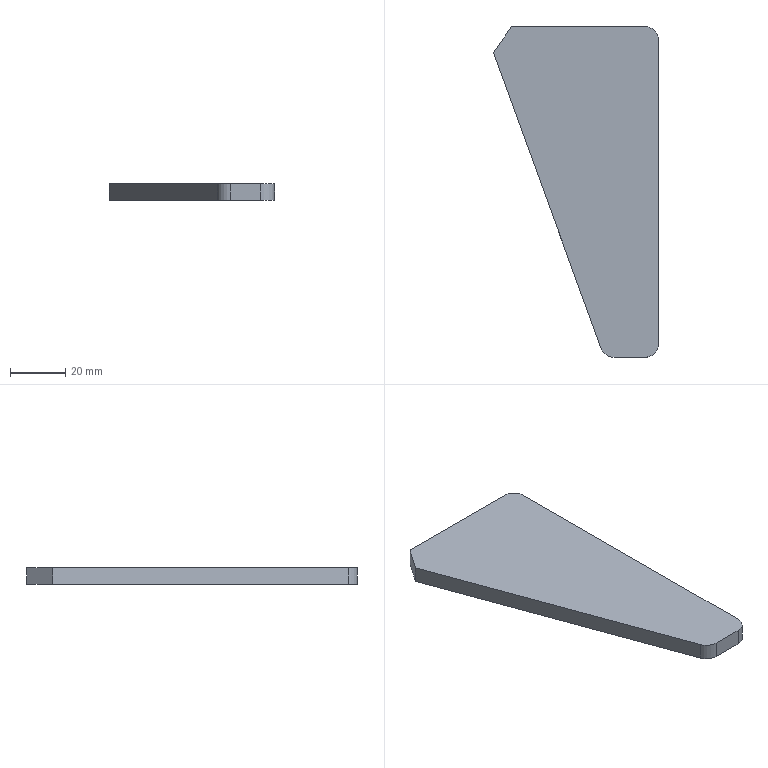Part | SolidWorks | features FlatPattern 1, SMBaseFlange 1, SheetMetal 1 | 1 solid | 10 faces | box 59.933 x 120 x 6 mm | volume 29531 mm3 | plane 7 | cylinder 3 | commonest cylinder face diameters 10 x3
STEP:
#1=CARTESIAN_POINT('',(295.827,-93.574,0.));
#2=VERTEX_POINT('',#1);
#3=CARTESIAN_POINT('',(290.827,-88.574,0.));
#4=VERTEX_POINT('',#3);
#5=CARTESIAN_POINT('',(290.827,-93.574,0.));
#6=DIRECTION('',(0.,0.,1.));
#7=DIRECTION('',(-1.,0.,0.));
#8=AXIS2_PLACEMENT_3D('',#5,#6,#7);
#9=CIRCLE('',#8,5.);
#10=EDGE_CURVE('',#2,#4,#9,.T.);
#11=ORIENTED_EDGE('',*,*,#10,.F.);
#12=CARTESIAN_POINT('',(295.827,-93.574,-6.));
#13=VERTEX_POINT('',#12);
#14=CARTESIAN_POINT('',(295.827,-93.574,-6.));
#15=DIRECTION('',(0.,0.,1.));
#16=VECTOR('',#15,1000.);
#17=LINE('',#14,#16);
#18=EDGE_CURVE('',#13,#2,#17,.T.);
#19=ORIENTED_EDGE('',*,*,#18,.F.);
#20=CARTESIAN_POINT('',(290.827,-88.574,-6.));
#21=VERTEX_POINT('',#20);
#22=CARTESIAN_POINT('',(290.827,-93.574,-6.));
#23=DIRECTION('',(0.,0.,1.));
#24=DIRECTION('',(-1.,0.,0.));
#25=AXIS2_PLACEMENT_3D('',#22,#23,#24);
#26=CIRCLE('',#25,5.);
#27=EDGE_CURVE('',#13,#21,#26,.T.);
#28=ORIENTED_EDGE('',*,*,#27,.T.);
#29=CARTESIAN_POINT('',(290.827,-88.574,-6.));
#30=DIRECTION('',(0.,0.,1.));
#31=VECTOR('',#30,1000.);
#32=LINE('',#29,#31);
#33=EDGE_CURVE('',#21,#4,#32,.T.);
#34=ORIENTED_EDGE('',*,*,#33,.T.);
#35=EDGE_LOOP('',(#11,#19,#28,#34));
#36=FACE_OUTER_BOUND('',#35,.T.);
#37=CARTESIAN_POINT('',(290.827,-93.574,-6.));
#38=DIRECTION('',(0.,0.,1.));
#39=DIRECTION('',(1.,0.,0.));
#40=AXIS2_PLACEMENT_3D('',#37,#38,#39);
#41=CYLINDRICAL_SURFACE('',#40,5.);
#42=ADVANCED_FACE('',(#36),#41,.T.);
#43=CARTESIAN_POINT('',(295.827,-203.574,0.));
#44=VERTEX_POINT('',#43);
#45=CARTESIAN_POINT('',(295.827,-93.574,0.));
#46=DIRECTION('',(0.,1.,0.));
#47=VECTOR('',#46,1000.);
#48=LINE('',#45,#47);
#49=EDGE_CURVE('',#44,#2,#48,.T.);
#50=ORIENTED_EDGE('',*,*,#49,.F.);
#51=CARTESIAN_POINT('',(295.827,-203.574,-6.));
#52=VERTEX_POINT('',#51);
#53=CARTESIAN_POINT('',(295.827,-203.574,-6.));
#54=DIRECTION('',(0.,0.,1.));
#55=VECTOR('',#54,1000.);
#56=LINE('',#53,#55);
#57=EDGE_CURVE('',#52,#44,#56,.T.);
#58=ORIENTED_EDGE('',*,*,#57,.F.);
#59=CARTESIAN_POINT('',(295.827,-93.574,-6.));
#60=DIRECTION('',(0.,1.,0.));
#61=VECTOR('',#60,1000.);
#62=LINE('',#59,#61);
#63=EDGE_CURVE('',#52,#13,#62,.T.);
#64=ORIENTED_EDGE('',*,*,#63,.T.);
#65=ORIENTED_EDGE('',*,*,#18,.T.);
#66=EDGE_LOOP('',(#50,#58,#64,#65));
#67=FACE_OUTER_BOUND('',#66,.T.);
#68=CARTESIAN_POINT('',(295.827,-93.574,-6.));
#69=DIRECTION('',(1.,0.,0.));
#70=DIRECTION('',(0.,0.,-1.));
#71=AXIS2_PLACEMENT_3D('',#68,#69,#70);
#72=PLANE('',#71);
#73=ADVANCED_FACE('',(#67),#72,.T.);
#74=CARTESIAN_POINT('',(290.827,-208.574,0.));
#75=VERTEX_POINT('',#74);
#76=CARTESIAN_POINT('',(290.827,-203.574,0.));
#77=DIRECTION('',(0.,0.,1.));
#78=DIRECTION('',(-1.,0.,0.));
#79=AXIS2_PLACEMENT_3D('',#76,#77,#78);
#80=CIRCLE('',#79,5.);
#81=EDGE_CURVE('',#75,#44,#80,.T.);
#82=ORIENTED_EDGE('',*,*,#81,.F.);
#83=CARTESIAN_POINT('',(290.827,-208.574,-6.));
#84=VERTEX_POINT('',#83);
#85=CARTESIAN_POINT('',(290.827,-208.574,-6.));
#86=DIRECTION('',(0.,0.,1.));
#87=VECTOR('',#86,1000.);
#88=LINE('',#85,#87);
#89=EDGE_CURVE('',#84,#75,#88,.T.);
#90=ORIENTED_EDGE('',*,*,#89,.F.);
#91=CARTESIAN_POINT('',(290.827,-203.574,-6.));
#92=DIRECTION('',(0.,0.,1.));
#93=DIRECTION('',(-1.,0.,0.));
#94=AXIS2_PLACEMENT_3D('',#91,#92,#93);
#95=CIRCLE('',#94,5.);
#96=EDGE_CURVE('',#84,#52,#95,.T.);
#97=ORIENTED_EDGE('',*,*,#96,.T.);
#98=ORIENTED_EDGE('',*,*,#57,.T.);
#99=EDGE_LOOP('',(#82,#90,#97,#98));
#100=FACE_OUTER_BOUND('',#99,.T.);
#101=CARTESIAN_POINT('',(290.827,-203.574,-6.));
#102=DIRECTION('',(0.,0.,1.));
#103=DIRECTION('',(1.,0.,0.));
#104=AXIS2_PLACEMENT_3D('',#101,#102,#103);
#105=CYLINDRICAL_SURFACE('',#104,5.);
#106=ADVANCED_FACE('',(#100),#105,.T.);
#107=CARTESIAN_POINT('',(279.652,-208.574,0.));
#108=VERTEX_POINT('',#107);
#109=CARTESIAN_POINT('',(290.827,-208.574,0.));
#110=DIRECTION('',(1.,0.,0.));
#111=VECTOR('',#110,1000.);
#112=LINE('',#109,#111);
#113=EDGE_CURVE('',#108,#75,#112,.T.);
#114=ORIENTED_EDGE('',*,*,#113,.F.);
#115=CARTESIAN_POINT('',(279.652,-208.574,-6.));
#116=VERTEX_POINT('',#115);
#117=CARTESIAN_POINT('',(279.652,-208.574,-6.));
#118=DIRECTION('',(0.,0.,1.));
#119=VECTOR('',#118,1000.);
#120=LINE('',#117,#119);
#121=EDGE_CURVE('',#116,#108,#120,.T.);
#122=ORIENTED_EDGE('',*,*,#121,.F.);
#123=CARTESIAN_POINT('',(290.827,-208.574,-6.));
#124=DIRECTION('',(1.,0.,0.));
#125=VECTOR('',#124,1000.);
#126=LINE('',#123,#125);
#127=EDGE_CURVE('',#116,#84,#126,.T.);
#128=ORIENTED_EDGE('',*,*,#127,.T.);
#129=ORIENTED_EDGE('',*,*,#89,.T.);
#130=EDGE_LOOP('',(#114,#122,#128,#129));
#131=FACE_OUTER_BOUND('',#130,.T.);
#132=CARTESIAN_POINT('',(290.827,-208.574,-6.));
#133=DIRECTION('',(0.,-1.,0.));
#134=DIRECTION('',(0.,0.,-1.));
#135=AXIS2_PLACEMENT_3D('',#132,#133,#134);
#136=PLANE('',#135);
#137=ADVANCED_FACE('',(#131),#136,.T.);
#138=CARTESIAN_POINT('',(274.953,-205.284,0.));
#139=VERTEX_POINT('',#138);
#140=CARTESIAN_POINT('',(279.652,-203.574,0.));
#141=DIRECTION('',(0.,0.,1.));
#142=DIRECTION('',(1.,0.,0.));
#143=AXIS2_PLACEMENT_3D('',#140,#141,#142);
#144=CIRCLE('',#143,5.);
#145=EDGE_CURVE('',#139,#108,#144,.T.);
#146=ORIENTED_EDGE('',*,*,#145,.F.);
#147=CARTESIAN_POINT('',(274.953,-205.284,-6.));
#148=VERTEX_POINT('',#147);
#149=CARTESIAN_POINT('',(274.953,-205.284,-6.));
#150=DIRECTION('',(0.,0.,1.));
#151=VECTOR('',#150,1000.);
#152=LINE('',#149,#151);
#153=EDGE_CURVE('',#148,#139,#152,.T.);
#154=ORIENTED_EDGE('',*,*,#153,.F.);
#155=CARTESIAN_POINT('',(279.652,-203.574,-6.));
#156=DIRECTION('',(0.,0.,1.));
#157=DIRECTION('',(1.,0.,0.));
#158=AXIS2_PLACEMENT_3D('',#155,#156,#157);
#159=CIRCLE('',#158,5.);
#160=EDGE_CURVE('',#148,#116,#159,.T.);
#161=ORIENTED_EDGE('',*,*,#160,.T.);
#162=ORIENTED_EDGE('',*,*,#121,.T.);
#163=EDGE_LOOP('',(#146,#154,#161,#162));
#164=FACE_OUTER_BOUND('',#163,.T.);
#165=CARTESIAN_POINT('',(279.652,-203.574,-6.));
#166=DIRECTION('',(0.,0.,1.));
#167=DIRECTION('',(1.,0.,0.));
#168=AXIS2_PLACEMENT_3D('',#165,#166,#167);
#169=CYLINDRICAL_SURFACE('',#168,5.);
#170=ADVANCED_FACE('',(#164),#169,.T.);
#171=CARTESIAN_POINT('',(235.894,-97.971,0.));
#172=VERTEX_POINT('',#171);
#173=CARTESIAN_POINT('',(274.953,-205.284,0.));
#174=DIRECTION('',(0.342,-0.9397,0.));
#175=VECTOR('',#174,1000.);
#176=LINE('',#173,#175);
#177=EDGE_CURVE('',#172,#139,#176,.T.);
#178=ORIENTED_EDGE('',*,*,#177,.F.);
#179=CARTESIAN_POINT('',(235.894,-97.971,-6.));
#180=VERTEX_POINT('',#179);
#181=CARTESIAN_POINT('',(235.894,-97.971,-6.));
#182=DIRECTION('',(0.,0.,1.));
#183=VECTOR('',#182,1000.);
#184=LINE('',#181,#183);
#185=EDGE_CURVE('',#180,#172,#184,.T.);
#186=ORIENTED_EDGE('',*,*,#185,.F.);
#187=CARTESIAN_POINT('',(274.953,-205.284,-6.));
#188=DIRECTION('',(0.342,-0.9397,0.));
#189=VECTOR('',#188,1000.);
#190=LINE('',#187,#189);
#191=EDGE_CURVE('',#180,#148,#190,.T.);
#192=ORIENTED_EDGE('',*,*,#191,.T.);
#193=ORIENTED_EDGE('',*,*,#153,.T.);
#194=EDGE_LOOP('',(#178,#186,#192,#193));
#195=FACE_OUTER_BOUND('',#194,.T.);
#196=CARTESIAN_POINT('',(274.953,-205.284,-6.));
#197=DIRECTION('',(-0.9397,-0.342,0.));
#198=DIRECTION('',(0.342,-0.9397,0.));
#199=AXIS2_PLACEMENT_3D('',#196,#197,#198);
#200=PLANE('',#199);
#201=ADVANCED_FACE('',(#195),#200,.T.);
#202=CARTESIAN_POINT('',(242.474,-88.574,0.));
#203=VERTEX_POINT('',#202);
#204=CARTESIAN_POINT('',(235.894,-97.971,0.));
#205=DIRECTION('',(-0.5736,-0.8192,0.));
#206=VECTOR('',#205,1000.);
#207=LINE('',#204,#206);
#208=EDGE_CURVE('',#203,#172,#207,.T.);
#209=ORIENTED_EDGE('',*,*,#208,.F.);
#210=CARTESIAN_POINT('',(242.474,-88.574,-6.));
#211=VERTEX_POINT('',#210);
#212=CARTESIAN_POINT('',(242.474,-88.574,-6.));
#213=DIRECTION('',(0.,0.,1.));
#214=VECTOR('',#213,1000.);
#215=LINE('',#212,#214);
#216=EDGE_CURVE('',#211,#203,#215,.T.);
#217=ORIENTED_EDGE('',*,*,#216,.F.);
#218=CARTESIAN_POINT('',(235.894,-97.971,-6.));
#219=DIRECTION('',(-0.5736,-0.8192,0.));
#220=VECTOR('',#219,1000.);
#221=LINE('',#218,#220);
#222=EDGE_CURVE('',#211,#180,#221,.T.);
#223=ORIENTED_EDGE('',*,*,#222,.T.);
#224=ORIENTED_EDGE('',*,*,#185,.T.);
#225=EDGE_LOOP('',(#209,#217,#223,#224));
#226=FACE_OUTER_BOUND('',#225,.T.);
#227=CARTESIAN_POINT('',(235.894,-97.971,-6.));
#228=DIRECTION('',(-0.8192,0.5736,0.));
#229=DIRECTION('',(-0.5736,-0.8192,0.));
#230=AXIS2_PLACEMENT_3D('',#227,#228,#229);
#231=PLANE('',#230);
#232=ADVANCED_FACE('',(#226),#231,.T.);
#233=CARTESIAN_POINT('',(242.474,-88.574,0.));
#234=DIRECTION('',(-1.,0.,0.));
#235=VECTOR('',#234,1000.);
#236=LINE('',#233,#235);
#237=EDGE_CURVE('',#4,#203,#236,.T.);
#238=ORIENTED_EDGE('',*,*,#237,.F.);
#239=ORIENTED_EDGE('',*,*,#33,.F.);
#240=CARTESIAN_POINT('',(242.474,-88.574,-6.));
#241=DIRECTION('',(-1.,0.,0.));
#242=VECTOR('',#241,1000.);
#243=LINE('',#240,#242);
#244=EDGE_CURVE('',#21,#211,#243,.T.);
#245=ORIENTED_EDGE('',*,*,#244,.T.);
#246=ORIENTED_EDGE('',*,*,#216,.T.);
#247=EDGE_LOOP('',(#238,#239,#245,#246));
#248=FACE_OUTER_BOUND('',#247,.T.);
#249=CARTESIAN_POINT('',(242.474,-88.574,-6.));
#250=DIRECTION('',(0.,1.,0.));
#251=DIRECTION('',(-1.,0.,0.));
#252=AXIS2_PLACEMENT_3D('',#249,#250,#251);
#253=PLANE('',#252);
#254=ADVANCED_FACE('',(#248),#253,.T.);
#255=ORIENTED_EDGE('',*,*,#27,.F.);
#256=ORIENTED_EDGE('',*,*,#63,.F.);
#257=ORIENTED_EDGE('',*,*,#96,.F.);
#258=ORIENTED_EDGE('',*,*,#127,.F.);
#259=ORIENTED_EDGE('',*,*,#160,.F.);
#260=ORIENTED_EDGE('',*,*,#191,.F.);
#261=ORIENTED_EDGE('',*,*,#222,.F.);
#262=ORIENTED_EDGE('',*,*,#244,.F.);
#263=EDGE_LOOP('',(#255,#256,#257,#258,#259,#260,#261,#262));
#264=FACE_OUTER_BOUND('',#263,.T.);
#265=CARTESIAN_POINT('',(290.827,-93.574,-6.));
#266=DIRECTION('',(0.,0.,-1.));
#267=DIRECTION('',(-1.,0.,0.));
#268=AXIS2_PLACEMENT_3D('',#265,#266,#267);
#269=PLANE('',#268);
#270=ADVANCED_FACE('',(#264),#269,.T.);
#271=ORIENTED_EDGE('',*,*,#10,.T.);
#272=ORIENTED_EDGE('',*,*,#237,.T.);
#273=ORIENTED_EDGE('',*,*,#208,.T.);
#274=ORIENTED_EDGE('',*,*,#177,.T.);
#275=ORIENTED_EDGE('',*,*,#145,.T.);
#276=ORIENTED_EDGE('',*,*,#113,.T.);
#277=ORIENTED_EDGE('',*,*,#81,.T.);
#278=ORIENTED_EDGE('',*,*,#49,.T.);
#279=EDGE_LOOP('',(#271,#272,#273,#274,#275,#276,#277,#278));
#280=FACE_OUTER_BOUND('',#279,.T.);
#281=CARTESIAN_POINT('',(290.827,-93.574,0.));
#282=DIRECTION('',(0.,0.,-1.));
#283=DIRECTION('',(-1.,0.,0.));
#284=AXIS2_PLACEMENT_3D('',#281,#282,#283);
#285=PLANE('',#284);
#286=ADVANCED_FACE('',(#280),#285,.F.);
#287=CLOSED_SHELL('',(#42,#73,#106,#137,#170,#201,#232,#254,#270,#286));
#288=MANIFOLD_SOLID_BREP('',#287);
#289=CARTESIAN_POINT('',(0.,0.,0.));
#290=DIRECTION('',(0.,0.,1.));
#291=DIRECTION('',(1.,0.,0.));
#292=AXIS2_PLACEMENT_3D('',#289,#290,#291);
#293=(LENGTH_UNIT()NAMED_UNIT(*)SI_UNIT(.MILLI.,.METRE.));
#294=UNCERTAINTY_MEASURE_WITH_UNIT(LENGTH_MEASURE(0.00001),#293,'','');
#295=(NAMED_UNIT(*)PLANE_ANGLE_UNIT()SI_UNIT($,.RADIAN.));
#296=(NAMED_UNIT(*)SI_UNIT($,.STERADIAN.)SOLID_ANGLE_UNIT());
#297=(GEOMETRIC_REPRESENTATION_CONTEXT(3)GLOBAL_UNCERTAINTY_ASSIGNED_CONTEXT((#294))GLOBAL_UNIT_ASSIGNED_CONTEXT((#293,#295,#296))REPRESENTATION_CONTEXT('',''));
#298=ADVANCED_BREP_SHAPE_REPRESENTATION('',(#288,#292),#297);